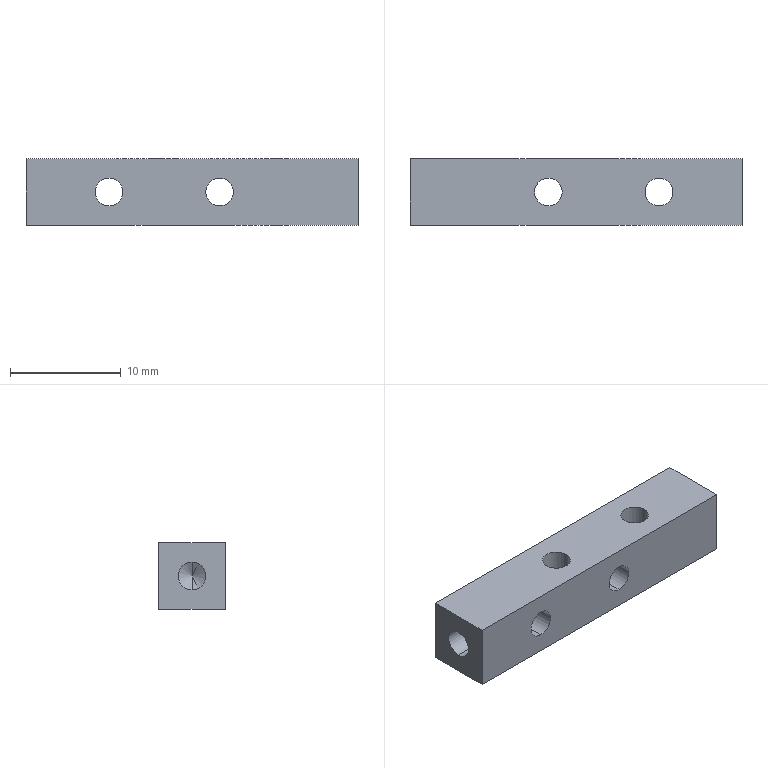Part | SolidWorks | features HoleWzd 4, Extrusion 1 | 1 solid | 22 faces | box 30 x 6 x 6 mm | volume 918.019 mm3 | cylinder 12 | plane 6 | cone 4 | commonest cylinder face diameters 2.5 x12
STEP:
#1=CARTESIAN_POINT('',(10.751,3.,1.25));
#2=VERTEX_POINT('',#1);
#3=CARTESIAN_POINT('',(10.751,3.,-1.25));
#4=VERTEX_POINT('',#3);
#5=CARTESIAN_POINT('',(10.751,3.,0.));
#6=DIRECTION('',(1.,0.,0.));
#7=DIRECTION('',(0.,0.,-1.));
#8=AXIS2_PLACEMENT_3D('',#5,#6,#7);
#9=CIRCLE('',#8,1.25);
#10=EDGE_CURVE('',#2,#4,#9,.T.);
#11=ORIENTED_EDGE('',*,*,#10,.F.);
#12=CARTESIAN_POINT('',(15.,3.,1.25));
#13=VERTEX_POINT('',#12);
#14=CARTESIAN_POINT('',(15.,3.,1.25));
#15=DIRECTION('',(1.,0.,0.));
#16=VECTOR('',#15,1000.);
#17=LINE('',#14,#16);
#18=EDGE_CURVE('',#2,#13,#17,.T.);
#19=ORIENTED_EDGE('',*,*,#18,.T.);
#20=CARTESIAN_POINT('',(15.,3.,-1.25));
#21=VERTEX_POINT('',#20);
#22=CARTESIAN_POINT('',(15.,3.,0.));
#23=DIRECTION('',(1.,0.,0.));
#24=DIRECTION('',(0.,0.,-1.));
#25=AXIS2_PLACEMENT_3D('',#22,#23,#24);
#26=CIRCLE('',#25,1.25);
#27=EDGE_CURVE('',#13,#21,#26,.T.);
#28=ORIENTED_EDGE('',*,*,#27,.T.);
#29=CARTESIAN_POINT('',(15.,3.,-1.25));
#30=DIRECTION('',(1.,0.,0.));
#31=VECTOR('',#30,1000.);
#32=LINE('',#29,#31);
#33=EDGE_CURVE('',#4,#21,#32,.T.);
#34=ORIENTED_EDGE('',*,*,#33,.F.);
#35=EDGE_LOOP('',(#11,#19,#28,#34));
#36=FACE_OUTER_BOUND('',#35,.T.);
#37=CARTESIAN_POINT('',(15.,3.,0.));
#38=DIRECTION('',(1.,0.,0.));
#39=DIRECTION('',(0.,0.,-1.));
#40=AXIS2_PLACEMENT_3D('',#37,#38,#39);
#41=CYLINDRICAL_SURFACE('',#40,1.25);
#42=ADVANCED_FACE('',(#36),#41,.F.);
#43=CARTESIAN_POINT('',(10.,3.,0.));
#44=VERTEX_POINT('',#43);
#45=CARTESIAN_POINT('',(10.751,3.,-1.25));
#46=DIRECTION('',(0.515,0.,-0.8572));
#47=VECTOR('',#46,1000.);
#48=LINE('',#45,#47);
#49=EDGE_CURVE('',#44,#4,#48,.T.);
#50=ORIENTED_EDGE('',*,*,#49,.F.);
#51=CARTESIAN_POINT('',(10.751,3.,1.25));
#52=DIRECTION('',(0.515,0.,0.8572));
#53=VECTOR('',#52,1000.);
#54=LINE('',#51,#53);
#55=EDGE_CURVE('',#44,#2,#54,.T.);
#56=ORIENTED_EDGE('',*,*,#55,.T.);
#57=ORIENTED_EDGE('',*,*,#10,.T.);
#58=EDGE_LOOP('',(#50,#56,#57));
#59=FACE_OUTER_BOUND('',#58,.T.);
#60=CARTESIAN_POINT('',(10.751,3.,0.));
#61=DIRECTION('',(1.,0.,0.));
#62=DIRECTION('',(0.,0.,-1.));
#63=AXIS2_PLACEMENT_3D('',#60,#61,#62);
#64=CONICAL_SURFACE('',#63,1.25,1.03);
#65=ADVANCED_FACE('',(#59),#64,.F.);
#66=CARTESIAN_POINT('',(-10.751,3.,-1.25));
#67=VERTEX_POINT('',#66);
#68=CARTESIAN_POINT('',(-10.751,3.,1.25));
#69=VERTEX_POINT('',#68);
#70=CARTESIAN_POINT('',(-10.751,3.,0.));
#71=DIRECTION('',(-1.,0.,0.));
#72=DIRECTION('',(0.,0.,1.));
#73=AXIS2_PLACEMENT_3D('',#70,#71,#72);
#74=CIRCLE('',#73,1.25);
#75=EDGE_CURVE('',#67,#69,#74,.T.);
#76=ORIENTED_EDGE('',*,*,#75,.F.);
#77=CARTESIAN_POINT('',(-15.,3.,-1.25));
#78=VERTEX_POINT('',#77);
#79=CARTESIAN_POINT('',(-15.,3.,-1.25));
#80=DIRECTION('',(-1.,0.,0.));
#81=VECTOR('',#80,1000.);
#82=LINE('',#79,#81);
#83=EDGE_CURVE('',#67,#78,#82,.T.);
#84=ORIENTED_EDGE('',*,*,#83,.T.);
#85=CARTESIAN_POINT('',(-15.,3.,1.25));
#86=VERTEX_POINT('',#85);
#87=CARTESIAN_POINT('',(-15.,3.,0.));
#88=DIRECTION('',(-1.,0.,0.));
#89=DIRECTION('',(0.,0.,1.));
#90=AXIS2_PLACEMENT_3D('',#87,#88,#89);
#91=CIRCLE('',#90,1.25);
#92=EDGE_CURVE('',#78,#86,#91,.T.);
#93=ORIENTED_EDGE('',*,*,#92,.T.);
#94=CARTESIAN_POINT('',(-15.,3.,1.25));
#95=DIRECTION('',(-1.,0.,0.));
#96=VECTOR('',#95,1000.);
#97=LINE('',#94,#96);
#98=EDGE_CURVE('',#69,#86,#97,.T.);
#99=ORIENTED_EDGE('',*,*,#98,.F.);
#100=EDGE_LOOP('',(#76,#84,#93,#99));
#101=FACE_OUTER_BOUND('',#100,.T.);
#102=CARTESIAN_POINT('',(-15.,3.,0.));
#103=DIRECTION('',(-1.,0.,0.));
#104=DIRECTION('',(0.,0.,1.));
#105=AXIS2_PLACEMENT_3D('',#102,#103,#104);
#106=CYLINDRICAL_SURFACE('',#105,1.25);
#107=ADVANCED_FACE('',(#101),#106,.F.);
#108=CARTESIAN_POINT('',(-10.,3.,0.));
#109=VERTEX_POINT('',#108);
#110=CARTESIAN_POINT('',(-10.751,3.,1.25));
#111=DIRECTION('',(-0.515,0.,0.8572));
#112=VECTOR('',#111,1000.);
#113=LINE('',#110,#112);
#114=EDGE_CURVE('',#109,#69,#113,.T.);
#115=ORIENTED_EDGE('',*,*,#114,.F.);
#116=CARTESIAN_POINT('',(-10.751,3.,-1.25));
#117=DIRECTION('',(-0.515,0.,-0.8572));
#118=VECTOR('',#117,1000.);
#119=LINE('',#116,#118);
#120=EDGE_CURVE('',#109,#67,#119,.T.);
#121=ORIENTED_EDGE('',*,*,#120,.T.);
#122=ORIENTED_EDGE('',*,*,#75,.T.);
#123=EDGE_LOOP('',(#115,#121,#122));
#124=FACE_OUTER_BOUND('',#123,.T.);
#125=CARTESIAN_POINT('',(-10.751,3.,0.));
#126=DIRECTION('',(-1.,0.,0.));
#127=DIRECTION('',(0.,0.,1.));
#128=AXIS2_PLACEMENT_3D('',#125,#126,#127);
#129=CONICAL_SURFACE('',#128,1.25,1.03);
#130=ADVANCED_FACE('',(#124),#129,.F.);
#131=CARTESIAN_POINT('',(-7.5,0.,-1.25));
#132=VERTEX_POINT('',#131);
#133=CARTESIAN_POINT('',(-7.5,0.,1.25));
#134=VERTEX_POINT('',#133);
#135=CARTESIAN_POINT('',(-7.5,0.,0.));
#136=DIRECTION('',(0.,1.,0.));
#137=DIRECTION('',(0.,0.,1.));
#138=AXIS2_PLACEMENT_3D('',#135,#136,#137);
#139=CIRCLE('',#138,1.25);
#140=EDGE_CURVE('',#132,#134,#139,.T.);
#141=ORIENTED_EDGE('',*,*,#140,.F.);
#142=CARTESIAN_POINT('',(-7.5,6.,-1.25));
#143=VERTEX_POINT('',#142);
#144=CARTESIAN_POINT('',(-7.5,6.,-1.25));
#145=DIRECTION('',(0.,1.,0.));
#146=VECTOR('',#145,1000.);
#147=LINE('',#144,#146);
#148=EDGE_CURVE('',#132,#143,#147,.T.);
#149=ORIENTED_EDGE('',*,*,#148,.T.);
#150=CARTESIAN_POINT('',(-7.5,6.,1.25));
#151=VERTEX_POINT('',#150);
#152=CARTESIAN_POINT('',(-7.5,6.,0.));
#153=DIRECTION('',(0.,1.,0.));
#154=DIRECTION('',(0.,0.,1.));
#155=AXIS2_PLACEMENT_3D('',#152,#153,#154);
#156=CIRCLE('',#155,1.25);
#157=EDGE_CURVE('',#143,#151,#156,.T.);
#158=ORIENTED_EDGE('',*,*,#157,.T.);
#159=CARTESIAN_POINT('',(-7.5,6.,1.25));
#160=DIRECTION('',(0.,1.,0.));
#161=VECTOR('',#160,1000.);
#162=LINE('',#159,#161);
#163=EDGE_CURVE('',#134,#151,#162,.T.);
#164=ORIENTED_EDGE('',*,*,#163,.F.);
#165=EDGE_LOOP('',(#141,#149,#158,#164));
#166=FACE_OUTER_BOUND('',#165,.T.);
#167=CARTESIAN_POINT('',(-7.5,6.,0.));
#168=DIRECTION('',(0.,1.,0.));
#169=DIRECTION('',(0.,0.,1.));
#170=AXIS2_PLACEMENT_3D('',#167,#168,#169);
#171=CYLINDRICAL_SURFACE('',#170,1.25);
#172=ADVANCED_FACE('',(#166),#171,.F.);
#173=CARTESIAN_POINT('',(2.5,0.,-1.25));
#174=VERTEX_POINT('',#173);
#175=CARTESIAN_POINT('',(2.5,0.,1.25));
#176=VERTEX_POINT('',#175);
#177=CARTESIAN_POINT('',(2.5,0.,0.));
#178=DIRECTION('',(0.,1.,0.));
#179=DIRECTION('',(0.,0.,1.));
#180=AXIS2_PLACEMENT_3D('',#177,#178,#179);
#181=CIRCLE('',#180,1.25);
#182=EDGE_CURVE('',#174,#176,#181,.T.);
#183=ORIENTED_EDGE('',*,*,#182,.F.);
#184=CARTESIAN_POINT('',(2.5,6.,-1.25));
#185=VERTEX_POINT('',#184);
#186=CARTESIAN_POINT('',(2.5,6.,-1.25));
#187=DIRECTION('',(0.,1.,0.));
#188=VECTOR('',#187,1000.);
#189=LINE('',#186,#188);
#190=EDGE_CURVE('',#174,#185,#189,.T.);
#191=ORIENTED_EDGE('',*,*,#190,.T.);
#192=CARTESIAN_POINT('',(2.5,6.,1.25));
#193=VERTEX_POINT('',#192);
#194=CARTESIAN_POINT('',(2.5,6.,0.));
#195=DIRECTION('',(0.,1.,0.));
#196=DIRECTION('',(0.,0.,1.));
#197=AXIS2_PLACEMENT_3D('',#194,#195,#196);
#198=CIRCLE('',#197,1.25);
#199=EDGE_CURVE('',#185,#193,#198,.T.);
#200=ORIENTED_EDGE('',*,*,#199,.T.);
#201=CARTESIAN_POINT('',(2.5,6.,1.25));
#202=DIRECTION('',(0.,1.,0.));
#203=VECTOR('',#202,1000.);
#204=LINE('',#201,#203);
#205=EDGE_CURVE('',#176,#193,#204,.T.);
#206=ORIENTED_EDGE('',*,*,#205,.F.);
#207=EDGE_LOOP('',(#183,#191,#200,#206));
#208=FACE_OUTER_BOUND('',#207,.T.);
#209=CARTESIAN_POINT('',(2.5,6.,0.));
#210=DIRECTION('',(0.,1.,0.));
#211=DIRECTION('',(0.,0.,1.));
#212=AXIS2_PLACEMENT_3D('',#209,#210,#211);
#213=CYLINDRICAL_SURFACE('',#212,1.25);
#214=ADVANCED_FACE('',(#208),#213,.F.);
#215=CARTESIAN_POINT('',(6.25,3.,-3.));
#216=VERTEX_POINT('',#215);
#217=CARTESIAN_POINT('',(8.75,3.,-3.));
#218=VERTEX_POINT('',#217);
#219=CARTESIAN_POINT('',(7.5,3.,-3.));
#220=DIRECTION('',(0.,0.,1.));
#221=DIRECTION('',(1.,0.,0.));
#222=AXIS2_PLACEMENT_3D('',#219,#220,#221);
#223=CIRCLE('',#222,1.25);
#224=EDGE_CURVE('',#216,#218,#223,.T.);
#225=ORIENTED_EDGE('',*,*,#224,.F.);
#226=CARTESIAN_POINT('',(6.25,3.,3.));
#227=VERTEX_POINT('',#226);
#228=CARTESIAN_POINT('',(6.25,3.,3.));
#229=DIRECTION('',(0.,0.,1.));
#230=VECTOR('',#229,1000.);
#231=LINE('',#228,#230);
#232=EDGE_CURVE('',#216,#227,#231,.T.);
#233=ORIENTED_EDGE('',*,*,#232,.T.);
#234=CARTESIAN_POINT('',(8.75,3.,3.));
#235=VERTEX_POINT('',#234);
#236=CARTESIAN_POINT('',(7.5,3.,3.));
#237=DIRECTION('',(0.,0.,1.));
#238=DIRECTION('',(1.,0.,0.));
#239=AXIS2_PLACEMENT_3D('',#236,#237,#238);
#240=CIRCLE('',#239,1.25);
#241=EDGE_CURVE('',#227,#235,#240,.T.);
#242=ORIENTED_EDGE('',*,*,#241,.T.);
#243=CARTESIAN_POINT('',(8.75,3.,3.));
#244=DIRECTION('',(0.,0.,1.));
#245=VECTOR('',#244,1000.);
#246=LINE('',#243,#245);
#247=EDGE_CURVE('',#218,#235,#246,.T.);
#248=ORIENTED_EDGE('',*,*,#247,.F.);
#249=EDGE_LOOP('',(#225,#233,#242,#248));
#250=FACE_OUTER_BOUND('',#249,.T.);
#251=CARTESIAN_POINT('',(7.5,3.,3.));
#252=DIRECTION('',(0.,0.,1.));
#253=DIRECTION('',(1.,0.,0.));
#254=AXIS2_PLACEMENT_3D('',#251,#252,#253);
#255=CYLINDRICAL_SURFACE('',#254,1.25);
#256=ADVANCED_FACE('',(#250),#255,.F.);
#257=CARTESIAN_POINT('',(-3.75,3.,-3.));
#258=VERTEX_POINT('',#257);
#259=CARTESIAN_POINT('',(-1.25,3.,-3.));
#260=VERTEX_POINT('',#259);
#261=CARTESIAN_POINT('',(-2.5,3.,-3.));
#262=DIRECTION('',(0.,0.,1.));
#263=DIRECTION('',(1.,0.,0.));
#264=AXIS2_PLACEMENT_3D('',#261,#262,#263);
#265=CIRCLE('',#264,1.25);
#266=EDGE_CURVE('',#258,#260,#265,.T.);
#267=ORIENTED_EDGE('',*,*,#266,.F.);
#268=CARTESIAN_POINT('',(-3.75,3.,3.));
#269=VERTEX_POINT('',#268);
#270=CARTESIAN_POINT('',(-3.75,3.,3.));
#271=DIRECTION('',(0.,0.,1.));
#272=VECTOR('',#271,1000.);
#273=LINE('',#270,#272);
#274=EDGE_CURVE('',#258,#269,#273,.T.);
#275=ORIENTED_EDGE('',*,*,#274,.T.);
#276=CARTESIAN_POINT('',(-1.25,3.,3.));
#277=VERTEX_POINT('',#276);
#278=CARTESIAN_POINT('',(-2.5,3.,3.));
#279=DIRECTION('',(0.,0.,1.));
#280=DIRECTION('',(1.,0.,0.));
#281=AXIS2_PLACEMENT_3D('',#278,#279,#280);
#282=CIRCLE('',#281,1.25);
#283=EDGE_CURVE('',#269,#277,#282,.T.);
#284=ORIENTED_EDGE('',*,*,#283,.T.);
#285=CARTESIAN_POINT('',(-1.25,3.,3.));
#286=DIRECTION('',(0.,0.,1.));
#287=VECTOR('',#286,1000.);
#288=LINE('',#285,#287);
#289=EDGE_CURVE('',#260,#277,#288,.T.);
#290=ORIENTED_EDGE('',*,*,#289,.F.);
#291=EDGE_LOOP('',(#267,#275,#284,#290));
#292=FACE_OUTER_BOUND('',#291,.T.);
#293=CARTESIAN_POINT('',(-2.5,3.,3.));
#294=DIRECTION('',(0.,0.,1.));
#295=DIRECTION('',(1.,0.,0.));
#296=AXIS2_PLACEMENT_3D('',#293,#294,#295);
#297=CYLINDRICAL_SURFACE('',#296,1.25);
#298=ADVANCED_FACE('',(#292),#297,.F.);
#299=CARTESIAN_POINT('',(-15.,3.,0.));
#300=DIRECTION('',(-1.,0.,0.));
#301=DIRECTION('',(0.,0.,1.));
#302=AXIS2_PLACEMENT_3D('',#299,#300,#301);
#303=CIRCLE('',#302,1.25);
#304=EDGE_CURVE('',#86,#78,#303,.T.);
#305=ORIENTED_EDGE('',*,*,#304,.F.);
#306=ORIENTED_EDGE('',*,*,#92,.F.);
#307=EDGE_LOOP('',(#305,#306));
#308=FACE_BOUND('',#307,.T.);
#309=CARTESIAN_POINT('',(-15.,0.,-3.));
#310=VERTEX_POINT('',#309);
#311=CARTESIAN_POINT('',(-15.,0.,3.));
#312=VERTEX_POINT('',#311);
#313=CARTESIAN_POINT('',(-15.,0.,3.));
#314=DIRECTION('',(0.,0.,1.));
#315=VECTOR('',#314,1000.);
#316=LINE('',#313,#315);
#317=EDGE_CURVE('',#310,#312,#316,.T.);
#318=ORIENTED_EDGE('',*,*,#317,.T.);
#319=CARTESIAN_POINT('',(-15.,6.,3.));
#320=VERTEX_POINT('',#319);
#321=CARTESIAN_POINT('',(-15.,6.,3.));
#322=DIRECTION('',(0.,-1.,0.));
#323=VECTOR('',#322,1000.);
#324=LINE('',#321,#323);
#325=EDGE_CURVE('',#320,#312,#324,.T.);
#326=ORIENTED_EDGE('',*,*,#325,.F.);
#327=CARTESIAN_POINT('',(-15.,6.,-3.));
#328=VERTEX_POINT('',#327);
#329=CARTESIAN_POINT('',(-15.,6.,3.));
#330=DIRECTION('',(0.,0.,1.));
#331=VECTOR('',#330,1000.);
#332=LINE('',#329,#331);
#333=EDGE_CURVE('',#328,#320,#332,.T.);
#334=ORIENTED_EDGE('',*,*,#333,.F.);
#335=CARTESIAN_POINT('',(-15.,6.,-3.));
#336=DIRECTION('',(0.,-1.,0.));
#337=VECTOR('',#336,1000.);
#338=LINE('',#335,#337);
#339=EDGE_CURVE('',#328,#310,#338,.T.);
#340=ORIENTED_EDGE('',*,*,#339,.T.);
#341=EDGE_LOOP('',(#318,#326,#334,#340));
#342=FACE_OUTER_BOUND('',#341,.T.);
#343=CARTESIAN_POINT('',(-15.,6.,3.));
#344=DIRECTION('',(1.,0.,0.));
#345=DIRECTION('',(0.,0.,-1.));
#346=AXIS2_PLACEMENT_3D('',#343,#344,#345);
#347=PLANE('',#346);
#348=ADVANCED_FACE('',(#308,#342),#347,.F.);
#349=CARTESIAN_POINT('',(7.5,3.,3.));
#350=DIRECTION('',(0.,0.,1.));
#351=DIRECTION('',(1.,0.,0.));
#352=AXIS2_PLACEMENT_3D('',#349,#350,#351);
#353=CIRCLE('',#352,1.25);
#354=EDGE_CURVE('',#235,#227,#353,.T.);
#355=ORIENTED_EDGE('',*,*,#354,.F.);
#356=ORIENTED_EDGE('',*,*,#241,.F.);
#357=EDGE_LOOP('',(#355,#356));
#358=FACE_BOUND('',#357,.T.);
#359=CARTESIAN_POINT('',(-2.5,3.,3.));
#360=DIRECTION('',(0.,0.,1.));
#361=DIRECTION('',(1.,0.,0.));
#362=AXIS2_PLACEMENT_3D('',#359,#360,#361);
#363=CIRCLE('',#362,1.25);
#364=EDGE_CURVE('',#277,#269,#363,.T.);
#365=ORIENTED_EDGE('',*,*,#364,.F.);
#366=ORIENTED_EDGE('',*,*,#283,.F.);
#367=EDGE_LOOP('',(#365,#366));
#368=FACE_BOUND('',#367,.T.);
#369=CARTESIAN_POINT('',(15.,0.,3.));
#370=VERTEX_POINT('',#369);
#371=CARTESIAN_POINT('',(15.,0.,3.));
#372=DIRECTION('',(1.,0.,0.));
#373=VECTOR('',#372,1000.);
#374=LINE('',#371,#373);
#375=EDGE_CURVE('',#312,#370,#374,.T.);
#376=ORIENTED_EDGE('',*,*,#375,.T.);
#377=CARTESIAN_POINT('',(15.,6.,3.));
#378=VERTEX_POINT('',#377);
#379=CARTESIAN_POINT('',(15.,6.,3.));
#380=DIRECTION('',(0.,-1.,0.));
#381=VECTOR('',#380,1000.);
#382=LINE('',#379,#381);
#383=EDGE_CURVE('',#378,#370,#382,.T.);
#384=ORIENTED_EDGE('',*,*,#383,.F.);
#385=CARTESIAN_POINT('',(15.,6.,3.));
#386=DIRECTION('',(1.,0.,0.));
#387=VECTOR('',#386,1000.);
#388=LINE('',#385,#387);
#389=EDGE_CURVE('',#320,#378,#388,.T.);
#390=ORIENTED_EDGE('',*,*,#389,.F.);
#391=ORIENTED_EDGE('',*,*,#325,.T.);
#392=EDGE_LOOP('',(#376,#384,#390,#391));
#393=FACE_OUTER_BOUND('',#392,.T.);
#394=CARTESIAN_POINT('',(15.,6.,3.));
#395=DIRECTION('',(0.,0.,-1.));
#396=DIRECTION('',(-1.,0.,0.));
#397=AXIS2_PLACEMENT_3D('',#394,#395,#396);
#398=PLANE('',#397);
#399=ADVANCED_FACE('',(#358,#368,#393),#398,.F.);
#400=CARTESIAN_POINT('',(15.,3.,0.));
#401=DIRECTION('',(1.,0.,0.));
#402=DIRECTION('',(0.,0.,-1.));
#403=AXIS2_PLACEMENT_3D('',#400,#401,#402);
#404=CIRCLE('',#403,1.25);
#405=EDGE_CURVE('',#21,#13,#404,.T.);
#406=ORIENTED_EDGE('',*,*,#405,.F.);
#407=ORIENTED_EDGE('',*,*,#27,.F.);
#408=EDGE_LOOP('',(#406,#407));
#409=FACE_BOUND('',#408,.T.);
#410=CARTESIAN_POINT('',(15.,0.,-3.));
#411=VERTEX_POINT('',#410);
#412=CARTESIAN_POINT('',(15.,0.,3.));
#413=DIRECTION('',(0.,0.,-1.));
#414=VECTOR('',#413,1000.);
#415=LINE('',#412,#414);
#416=EDGE_CURVE('',#370,#411,#415,.T.);
#417=ORIENTED_EDGE('',*,*,#416,.T.);
#418=CARTESIAN_POINT('',(15.,6.,-3.));
#419=VERTEX_POINT('',#418);
#420=CARTESIAN_POINT('',(15.,6.,-3.));
#421=DIRECTION('',(0.,-1.,0.));
#422=VECTOR('',#421,1000.);
#423=LINE('',#420,#422);
#424=EDGE_CURVE('',#419,#411,#423,.T.);
#425=ORIENTED_EDGE('',*,*,#424,.F.);
#426=CARTESIAN_POINT('',(15.,6.,3.));
#427=DIRECTION('',(0.,0.,-1.));
#428=VECTOR('',#427,1000.);
#429=LINE('',#426,#428);
#430=EDGE_CURVE('',#378,#419,#429,.T.);
#431=ORIENTED_EDGE('',*,*,#430,.F.);
#432=ORIENTED_EDGE('',*,*,#383,.T.);
#433=EDGE_LOOP('',(#417,#425,#431,#432));
#434=FACE_OUTER_BOUND('',#433,.T.);
#435=CARTESIAN_POINT('',(15.,6.,3.));
#436=DIRECTION('',(-1.,0.,0.));
#437=DIRECTION('',(0.,0.,1.));
#438=AXIS2_PLACEMENT_3D('',#435,#436,#437);
#439=PLANE('',#438);
#440=ADVANCED_FACE('',(#409,#434),#439,.F.);
#441=CARTESIAN_POINT('',(7.5,3.,-3.));
#442=DIRECTION('',(0.,0.,1.));
#443=DIRECTION('',(1.,0.,0.));
#444=AXIS2_PLACEMENT_3D('',#441,#442,#443);
#445=CIRCLE('',#444,1.25);
#446=EDGE_CURVE('',#218,#216,#445,.T.);
#447=ORIENTED_EDGE('',*,*,#446,.T.);
#448=ORIENTED_EDGE('',*,*,#224,.T.);
#449=EDGE_LOOP('',(#447,#448));
#450=FACE_BOUND('',#449,.T.);
#451=CARTESIAN_POINT('',(-2.5,3.,-3.));
#452=DIRECTION('',(0.,0.,1.));
#453=DIRECTION('',(1.,0.,0.));
#454=AXIS2_PLACEMENT_3D('',#451,#452,#453);
#455=CIRCLE('',#454,1.25);
#456=EDGE_CURVE('',#260,#258,#455,.T.);
#457=ORIENTED_EDGE('',*,*,#456,.T.);
#458=ORIENTED_EDGE('',*,*,#266,.T.);
#459=EDGE_LOOP('',(#457,#458));
#460=FACE_BOUND('',#459,.T.);
#461=CARTESIAN_POINT('',(15.,0.,-3.));
#462=DIRECTION('',(-1.,0.,0.));
#463=VECTOR('',#462,1000.);
#464=LINE('',#461,#463);
#465=EDGE_CURVE('',#411,#310,#464,.T.);
#466=ORIENTED_EDGE('',*,*,#465,.T.);
#467=ORIENTED_EDGE('',*,*,#339,.F.);
#468=CARTESIAN_POINT('',(15.,6.,-3.));
#469=DIRECTION('',(-1.,0.,0.));
#470=VECTOR('',#469,1000.);
#471=LINE('',#468,#470);
#472=EDGE_CURVE('',#419,#328,#471,.T.);
#473=ORIENTED_EDGE('',*,*,#472,.F.);
#474=ORIENTED_EDGE('',*,*,#424,.T.);
#475=EDGE_LOOP('',(#466,#467,#473,#474));
#476=FACE_OUTER_BOUND('',#475,.T.);
#477=CARTESIAN_POINT('',(15.,6.,-3.));
#478=DIRECTION('',(0.,0.,1.));
#479=DIRECTION('',(1.,0.,0.));
#480=AXIS2_PLACEMENT_3D('',#477,#478,#479);
#481=PLANE('',#480);
#482=ADVANCED_FACE('',(#450,#460,#476),#481,.F.);
#483=CARTESIAN_POINT('',(-7.5,6.,0.));
#484=DIRECTION('',(0.,1.,0.));
#485=DIRECTION('',(0.,0.,1.));
#486=AXIS2_PLACEMENT_3D('',#483,#484,#485);
#487=CIRCLE('',#486,1.25);
#488=EDGE_CURVE('',#151,#143,#487,.T.);
#489=ORIENTED_EDGE('',*,*,#488,.F.);
#490=ORIENTED_EDGE('',*,*,#157,.F.);
#491=EDGE_LOOP('',(#489,#490));
#492=FACE_BOUND('',#491,.T.);
#493=CARTESIAN_POINT('',(2.5,6.,0.));
#494=DIRECTION('',(0.,1.,0.));
#495=DIRECTION('',(0.,0.,1.));
#496=AXIS2_PLACEMENT_3D('',#493,#494,#495);
#497=CIRCLE('',#496,1.25);
#498=EDGE_CURVE('',#193,#185,#497,.T.);
#499=ORIENTED_EDGE('',*,*,#498,.F.);
#500=ORIENTED_EDGE('',*,*,#199,.F.);
#501=EDGE_LOOP('',(#499,#500));
#502=FACE_BOUND('',#501,.T.);
#503=ORIENTED_EDGE('',*,*,#333,.T.);
#504=ORIENTED_EDGE('',*,*,#389,.T.);
#505=ORIENTED_EDGE('',*,*,#430,.T.);
#506=ORIENTED_EDGE('',*,*,#472,.T.);
#507=EDGE_LOOP('',(#503,#504,#505,#506));
#508=FACE_OUTER_BOUND('',#507,.T.);
#509=CARTESIAN_POINT('',(0.,6.,0.));
#510=DIRECTION('',(0.,1.,0.));
#511=DIRECTION('',(0.,0.,1.));
#512=AXIS2_PLACEMENT_3D('',#509,#510,#511);
#513=PLANE('',#512);
#514=ADVANCED_FACE('',(#492,#502,#508),#513,.T.);
#515=CARTESIAN_POINT('',(-7.5,0.,0.));
#516=DIRECTION('',(0.,1.,0.));
#517=DIRECTION('',(0.,0.,1.));
#518=AXIS2_PLACEMENT_3D('',#515,#516,#517);
#519=CIRCLE('',#518,1.25);
#520=EDGE_CURVE('',#134,#132,#519,.T.);
#521=ORIENTED_EDGE('',*,*,#520,.T.);
#522=ORIENTED_EDGE('',*,*,#140,.T.);
#523=EDGE_LOOP('',(#521,#522));
#524=FACE_BOUND('',#523,.T.);
#525=CARTESIAN_POINT('',(2.5,0.,0.));
#526=DIRECTION('',(0.,1.,0.));
#527=DIRECTION('',(0.,0.,1.));
#528=AXIS2_PLACEMENT_3D('',#525,#526,#527);
#529=CIRCLE('',#528,1.25);
#530=EDGE_CURVE('',#176,#174,#529,.T.);
#531=ORIENTED_EDGE('',*,*,#530,.T.);
#532=ORIENTED_EDGE('',*,*,#182,.T.);
#533=EDGE_LOOP('',(#531,#532));
#534=FACE_BOUND('',#533,.T.);
#535=ORIENTED_EDGE('',*,*,#317,.F.);
#536=ORIENTED_EDGE('',*,*,#465,.F.);
#537=ORIENTED_EDGE('',*,*,#416,.F.);
#538=ORIENTED_EDGE('',*,*,#375,.F.);
#539=EDGE_LOOP('',(#535,#536,#537,#538));
#540=FACE_OUTER_BOUND('',#539,.T.);
#541=CARTESIAN_POINT('',(0.,0.,0.));
#542=DIRECTION('',(0.,1.,0.));
#543=DIRECTION('',(0.,0.,1.));
#544=AXIS2_PLACEMENT_3D('',#541,#542,#543);
#545=PLANE('',#544);
#546=ADVANCED_FACE('',(#524,#534,#540),#545,.F.);
#547=ORIENTED_EDGE('',*,*,#274,.F.);
#548=ORIENTED_EDGE('',*,*,#456,.F.);
#549=ORIENTED_EDGE('',*,*,#289,.T.);
#550=ORIENTED_EDGE('',*,*,#364,.T.);
#551=EDGE_LOOP('',(#547,#548,#549,#550));
#552=FACE_OUTER_BOUND('',#551,.T.);
#553=CARTESIAN_POINT('',(-2.5,3.,3.));
#554=DIRECTION('',(0.,0.,1.));
#555=DIRECTION('',(1.,0.,0.));
#556=AXIS2_PLACEMENT_3D('',#553,#554,#555);
#557=CYLINDRICAL_SURFACE('',#556,1.25);
#558=ADVANCED_FACE('',(#552),#557,.F.);
#559=ORIENTED_EDGE('',*,*,#232,.F.);
#560=ORIENTED_EDGE('',*,*,#446,.F.);
#561=ORIENTED_EDGE('',*,*,#247,.T.);
#562=ORIENTED_EDGE('',*,*,#354,.T.);
#563=EDGE_LOOP('',(#559,#560,#561,#562));
#564=FACE_OUTER_BOUND('',#563,.T.);
#565=CARTESIAN_POINT('',(7.5,3.,3.));
#566=DIRECTION('',(0.,0.,1.));
#567=DIRECTION('',(1.,0.,0.));
#568=AXIS2_PLACEMENT_3D('',#565,#566,#567);
#569=CYLINDRICAL_SURFACE('',#568,1.25);
#570=ADVANCED_FACE('',(#564),#569,.F.);
#571=ORIENTED_EDGE('',*,*,#190,.F.);
#572=ORIENTED_EDGE('',*,*,#530,.F.);
#573=ORIENTED_EDGE('',*,*,#205,.T.);
#574=ORIENTED_EDGE('',*,*,#498,.T.);
#575=EDGE_LOOP('',(#571,#572,#573,#574));
#576=FACE_OUTER_BOUND('',#575,.T.);
#577=CARTESIAN_POINT('',(2.5,6.,0.));
#578=DIRECTION('',(0.,1.,0.));
#579=DIRECTION('',(0.,0.,1.));
#580=AXIS2_PLACEMENT_3D('',#577,#578,#579);
#581=CYLINDRICAL_SURFACE('',#580,1.25);
#582=ADVANCED_FACE('',(#576),#581,.F.);
#583=ORIENTED_EDGE('',*,*,#148,.F.);
#584=ORIENTED_EDGE('',*,*,#520,.F.);
#585=ORIENTED_EDGE('',*,*,#163,.T.);
#586=ORIENTED_EDGE('',*,*,#488,.T.);
#587=EDGE_LOOP('',(#583,#584,#585,#586));
#588=FACE_OUTER_BOUND('',#587,.T.);
#589=CARTESIAN_POINT('',(-7.5,6.,0.));
#590=DIRECTION('',(0.,1.,0.));
#591=DIRECTION('',(0.,0.,1.));
#592=AXIS2_PLACEMENT_3D('',#589,#590,#591);
#593=CYLINDRICAL_SURFACE('',#592,1.25);
#594=ADVANCED_FACE('',(#588),#593,.F.);
#595=ORIENTED_EDGE('',*,*,#120,.F.);
#596=ORIENTED_EDGE('',*,*,#114,.T.);
#597=CARTESIAN_POINT('',(-10.751,3.,0.));
#598=DIRECTION('',(-1.,0.,0.));
#599=DIRECTION('',(0.,0.,1.));
#600=AXIS2_PLACEMENT_3D('',#597,#598,#599);
#601=CIRCLE('',#600,1.25);
#602=EDGE_CURVE('',#69,#67,#601,.T.);
#603=ORIENTED_EDGE('',*,*,#602,.T.);
#604=EDGE_LOOP('',(#595,#596,#603));
#605=FACE_OUTER_BOUND('',#604,.T.);
#606=CARTESIAN_POINT('',(-10.751,3.,0.));
#607=DIRECTION('',(-1.,0.,0.));
#608=DIRECTION('',(0.,0.,1.));
#609=AXIS2_PLACEMENT_3D('',#606,#607,#608);
#610=CONICAL_SURFACE('',#609,1.25,1.03);
#611=ADVANCED_FACE('',(#605),#610,.F.);
#612=ORIENTED_EDGE('',*,*,#83,.F.);
#613=ORIENTED_EDGE('',*,*,#602,.F.);
#614=ORIENTED_EDGE('',*,*,#98,.T.);
#615=ORIENTED_EDGE('',*,*,#304,.T.);
#616=EDGE_LOOP('',(#612,#613,#614,#615));
#617=FACE_OUTER_BOUND('',#616,.T.);
#618=CARTESIAN_POINT('',(-15.,3.,0.));
#619=DIRECTION('',(-1.,0.,0.));
#620=DIRECTION('',(0.,0.,1.));
#621=AXIS2_PLACEMENT_3D('',#618,#619,#620);
#622=CYLINDRICAL_SURFACE('',#621,1.25);
#623=ADVANCED_FACE('',(#617),#622,.F.);
#624=ORIENTED_EDGE('',*,*,#55,.F.);
#625=ORIENTED_EDGE('',*,*,#49,.T.);
#626=CARTESIAN_POINT('',(10.751,3.,0.));
#627=DIRECTION('',(1.,0.,0.));
#628=DIRECTION('',(0.,0.,-1.));
#629=AXIS2_PLACEMENT_3D('',#626,#627,#628);
#630=CIRCLE('',#629,1.25);
#631=EDGE_CURVE('',#4,#2,#630,.T.);
#632=ORIENTED_EDGE('',*,*,#631,.T.);
#633=EDGE_LOOP('',(#624,#625,#632));
#634=FACE_OUTER_BOUND('',#633,.T.);
#635=CARTESIAN_POINT('',(10.751,3.,0.));
#636=DIRECTION('',(1.,0.,0.));
#637=DIRECTION('',(0.,0.,-1.));
#638=AXIS2_PLACEMENT_3D('',#635,#636,#637);
#639=CONICAL_SURFACE('',#638,1.25,1.03);
#640=ADVANCED_FACE('',(#634),#639,.F.);
#641=ORIENTED_EDGE('',*,*,#18,.F.);
#642=ORIENTED_EDGE('',*,*,#631,.F.);
#643=ORIENTED_EDGE('',*,*,#33,.T.);
#644=ORIENTED_EDGE('',*,*,#405,.T.);
#645=EDGE_LOOP('',(#641,#642,#643,#644));
#646=FACE_OUTER_BOUND('',#645,.T.);
#647=CARTESIAN_POINT('',(15.,3.,0.));
#648=DIRECTION('',(1.,0.,0.));
#649=DIRECTION('',(0.,0.,-1.));
#650=AXIS2_PLACEMENT_3D('',#647,#648,#649);
#651=CYLINDRICAL_SURFACE('',#650,1.25);
#652=ADVANCED_FACE('',(#646),#651,.F.);
#653=CLOSED_SHELL('',(#42,#65,#107,#130,#172,#214,#256,#298,#348,#399,#440,#482,#514,#546,#558,#570,#582,#594,#611,#623,#640,#652));
#654=MANIFOLD_SOLID_BREP('',#653);
#655=CARTESIAN_POINT('',(0.,0.,0.));
#656=DIRECTION('',(0.,0.,1.));
#657=DIRECTION('',(1.,0.,0.));
#658=AXIS2_PLACEMENT_3D('',#655,#656,#657);
#659=(LENGTH_UNIT()NAMED_UNIT(*)SI_UNIT(.MILLI.,.METRE.));
#660=UNCERTAINTY_MEASURE_WITH_UNIT(LENGTH_MEASURE(0.00001),#659,'','');
#661=(NAMED_UNIT(*)PLANE_ANGLE_UNIT()SI_UNIT($,.RADIAN.));
#662=(NAMED_UNIT(*)SI_UNIT($,.STERADIAN.)SOLID_ANGLE_UNIT());
#663=(GEOMETRIC_REPRESENTATION_CONTEXT(3)GLOBAL_UNCERTAINTY_ASSIGNED_CONTEXT((#660))GLOBAL_UNIT_ASSIGNED_CONTEXT((#659,#661,#662))REPRESENTATION_CONTEXT('',''));
#664=ADVANCED_BREP_SHAPE_REPRESENTATION('',(#654,#658),#663);